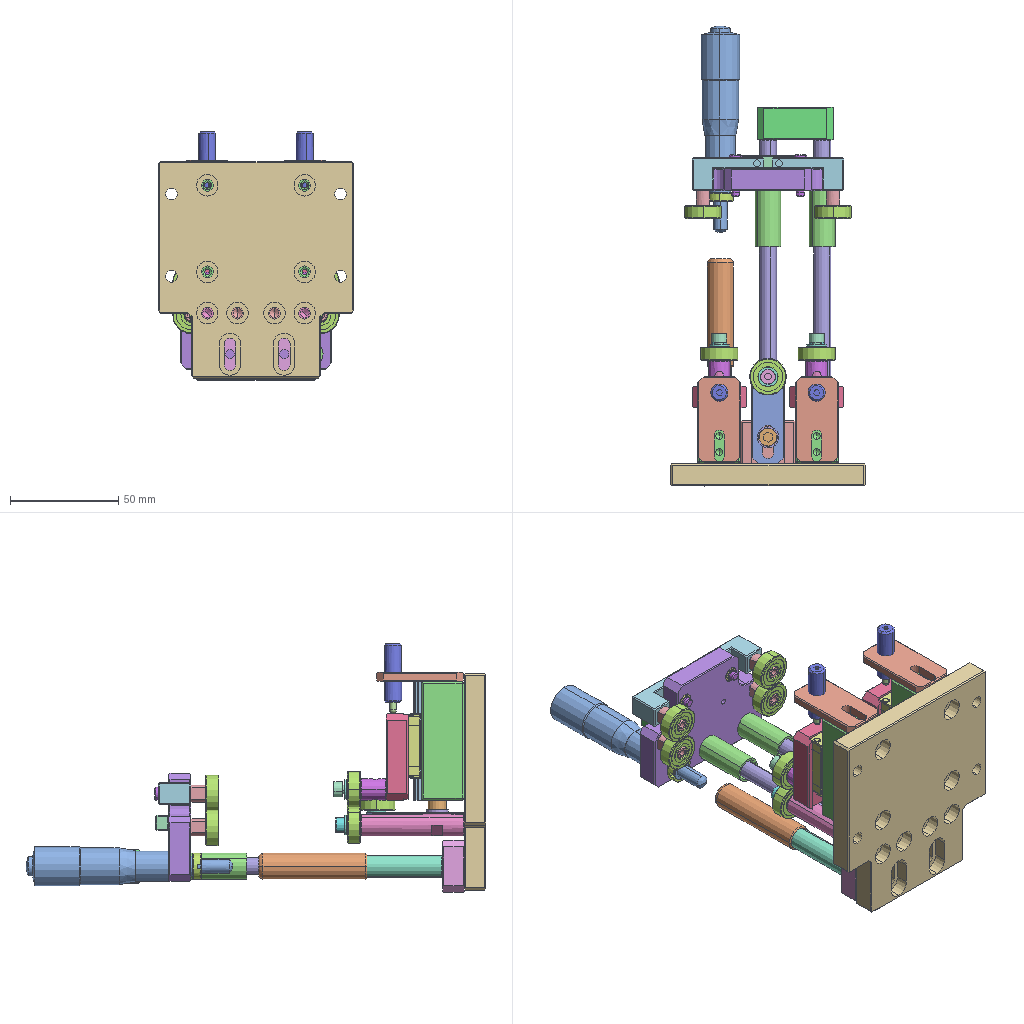Assembly | SolidWorks | 45 different items | 86 placed | box 90 x 212 x 115 mm
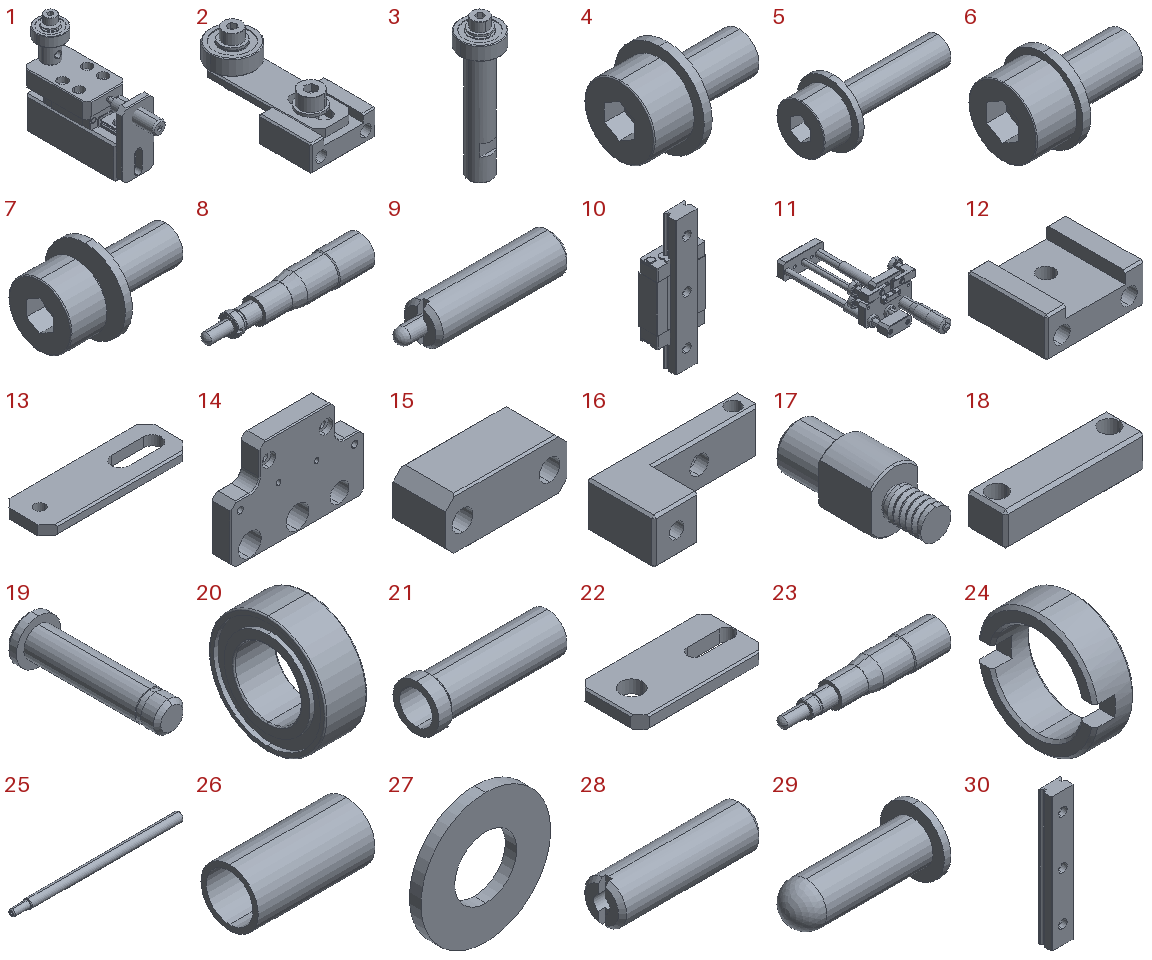Parts list (item | name | quantity | parent item | size | volume | features):
1 | (subassembly) | x2 | - | 25 x 75.736 x 60.345 mm | 39724 mm3 | -
2 | (subassembly) | x1 | - | 25 x 50.976 x 21.6 mm | 7360 mm3 | -
3 | (subassembly) | x2 | - | 17 x 17 x 59.3 mm | 5007 mm3 | -
4 | (subassembly) | x2 | in 3 | 12 x 9 x 9 mm | 278.436 mm3 | -
5 | (subassembly) | x1 | in 2 | 20 x 9 x 9 mm | 378.967 mm3 | -
6 | (subassembly) | x1 | in 2 | 15 x 10 x 10 mm | 502.571 mm3 | -
7 | (subassembly) | x2 | in 1 | 14 x 9 x 9 mm | 303.569 mm3 | -
8 | (subassembly) | x1 | in 11 | 95.5 x 18 x 18 mm | 15301 mm3 | -
9 | (subassembly) | x2 | in 1 | 32 x 8 x 8 mm | 1008 mm3 | -
10 | (subassembly) | x2 | in 1 | 20 x 10 x 55 mm | 5673 mm3 | -
11 | (subassembly) | x1 | - | 77 x 202.46 x 55 mm | 99143 mm3 | features CompositeCurve 4, MateUpdatePoint 3
12 | - | x1 | in 2 | 25 x 20 x 10 mm | 3625 mm3 | features HoleWzd 2, Chamfer 1, Extrusion 1, ICE 1
13 | - | x1 | in 2 | 45 x 15 x 3 mm | 1689 mm3 | features Chamfer 2, Extrusion 1, HoleWzd 1, ICE 1
14 | - | x1 | in 11 | 70 x 10 x 50 mm | 24960 mm3 | features ICE 5, Chamfer 3, HoleWzd 2, Cut 1, Extrusion 1, Fillet 1
15 | - | x1 | in 11 | 35 x 15 x 15 mm | 6742 mm3 | features Chamfer 2, Extrusion 1, ICE 1
16 | - | x2 | in 11 | 33 x 15 x 10 mm | 2355 mm3 | features ICE 5, Chamfer 1, Extrusion 1, HoleWzd 1, MirrorPattern 1
17 | - | x4 | in 11 | 6 x 18.5 x 8 mm | 437.837 mm3 | features ICE 4, Chamfer 2, Extrusion 1, Helix 1, HoleWzd 1, SweepCut 1
18 | - | x1 | in 11 | 25 x 7 x 6 mm | 851.742 mm3 | features HoleWzd 2, Chamfer 1, Extrusion 1
19 | - | x2 | in 11 | 6 x 19.5 x 6 mm | 263.49 mm3 | features Chamfer 2, Extrusion 1, ICE 1, RevCut 1
20 | - | x4 | in 11 | 2.5 x 7 x 7 mm | 58.917 mm3 | features RefAxis 6, 3DProfileFeature 2, Revolution 1
21 | - | x2 | in 11 | 40 x 14 x 14 mm | 1542 mm3 | features RefAxis 3, 3DProfileFeature 1, Revolution 1
22 | - | x2 | in 1 | 40 x 20 x 4 mm | 2715 mm3 | features Chamfer 2, Extrusion 1, HoleWzd 1, ICE 1
23 | - | x1 | in 8 | 95.5 x 18 x 18 mm | 15118 mm3 | features RefAxis 9, 3DProfileFeature 3, RevCut 1, Revolution 1
24 | - | x1 | in 8 | 4 x 12 x 12 mm | 182.884 mm3 | features RefAxis 3, 3DProfileFeature 1, ICE 1, Revolution 1
25 | - | x2 | in 11 | 155 x 8 x 8 mm | 7283 mm3 | features BaseBody 1, MoveFace 1
26 | - | x2 | in 11 | 20 x 9.8 x 9.8 mm | 503.283 mm3 | features RefAxis 3, 3DProfileFeature 1, Revolution 1
27 | - | x6 | in 2, 4, 5, 7 | 9 x 0.8 x 9 mm | 39.276 mm3 | features Revolution 1
28 | - | x2 | in 9 | 27 x 8 x 8 mm | 931.32 mm3 | features BaseBody 1
29 | - | x2 | in 9 | 10 x 4.8 x 4.8 mm | 76.851 mm3 | features BaseBody 1
30 | - | x2 | in 10 | 9 x 5.5 x 55 mm | 2182 mm3 | features BaseBody 1
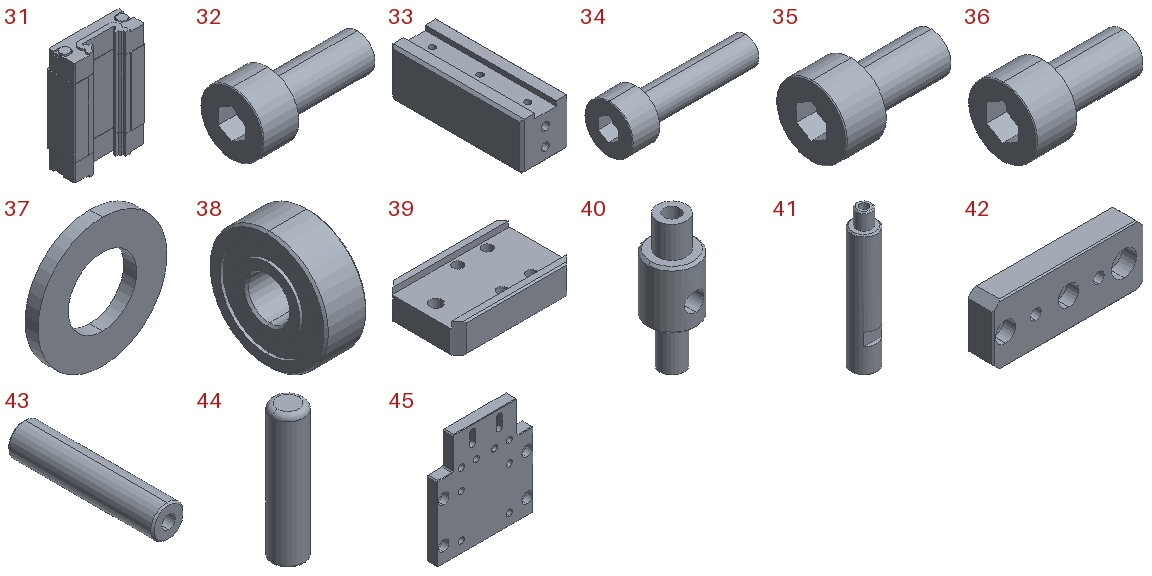31 | - | x2 | in 10 | 20 x 7.8 x 30 mm | 3491 mm3 | features BaseBody 1
32 | - | x2 | in 7 | 14 x 7 x 7 mm | 264.293 mm3 | features BlendCut 1, Cut 1, Fillet 1, LPattern 1, RevCut 1, Revolution 1
33 | - | x2 | in 1 | 20 x 55 x 20 mm | 20279 mm3 | features HoleWzd 3, Chamfer 1, Extrusion 1, ICE 1
34 | - | x1 | in 5 | 20 x 7 x 7 mm | 339.691 mm3 | features BlendCut 1, Cut 1, Fillet 1, LPattern 1, RevCut 1, Revolution 1
35 | - | x2 | in 4 | 12 x 7 x 7 mm | 239.16 mm3 | features BlendCut 1, Cut 1, Fillet 1, LPattern 1, RevCut 1, Revolution 1
36 | - | x1 | in 6 | 15 x 8.5 x 8.5 mm | 446.093 mm3 | features BlendCut 1, Cut 1, Fillet 1, LPattern 1, RevCut 1, Revolution 1
37 | - | x1 | in 6 | 10 x 1 x 10 mm | 56.478 mm3 | features Revolution 1
38 | - | x9 | in 1, 2, 3, 11 | 6 x 17 x 17 mm | 1125 mm3 | features BaseBody 1
39 | - | x2 | in 1 | 40 x 25 x 10 mm | 7537 mm3 | features Chamfer 2, HoleWzd 2, Extrusion 1, ICE 1
40 | - | x2 | in 1 | 10 x 10 x 27.5 mm | 1083 mm3 | features ICE 3, Chamfer 1, Extrusion 1, HoleWzd 1
41 | - | x2 | in 3 | 10 x 10 x 54.5 mm | 3603 mm3 | features HoleWzd 2, ICE 2, Chamfer 1, Extrusion 1, MirrorPattern 1
42 | - | x1 | in 11 | 60 x 10 x 24 mm | 12723 mm3 | features HoleWzd 4, Chamfer 2, Extrusion 1, ICE 1
43 | - | x1 | in 11 | 10 x 45 x 10 mm | 3349 mm3 | features 3DProfileFeature 1, Chamfer 1, Extrusion 1, HoleWzd 1
44 | - | x1 | in 11 | 12 x 12 x 50 mm | 4836 mm3 | features Fillet 2, Extrusion 1, ICE 1
45 | - | x1 | - | 90 x 10 x 100 mm | 71659 mm3 | features HoleWzd 5, Chamfer 2, ICE 2, Extrusion 1
Mates (type | each side: item.copy, entity, surface, feature):
In the top assembly
Coincident | 41.1 face plane Boss-Extrude1 | 45.1 face plane Boss-Extrude1
Coincident | 41.2 face plane Boss-Extrude1 | 45.1 face plane Boss-Extrude1
Width | 12.1 face plane Boss-Extrude1 | 12.1 face plane Boss-Extrude1 | 33.1 face plane Boss-Extrude1 | 33.2 face plane Boss-Extrude1
Coincident | 12.1 face plane Boss-Extrude1 | 45.1 face plane Boss-Extrude1
Coincident | 33.2 face plane Boss-Extrude1 | 45.1 face plane Boss-Extrude1
Coincident | 45.1 face plane Boss-Extrude1 | 42.1 face plane Boss-Extrude1
Parallel | 41.1 face cylinder M5 Tapped Hole1 | 45.1 face cylinder Hole Size (Based On) Socket Head Cap Screw Type2
Concentric | 41.1 face cylinder M5 Tapped Hole1 | 45.1 face cylinder Hole Size (Based On) Socket Head Cap Screw Type2
Concentric | 41.2 face cylinder M5 Tapped Hole1 | 45.1 face cylinder Hole Size (Based On) Socket Head Cap Screw Type2
Concentric | 12.1 face cylinder M5 Tapped Hole2 | 45.1 face cylinder Hole Size (Based On) Socket Head Cap Screw Type2 | 2 times
Concentric | 33.2 face cylinder M5 Tapped Hole1 | 45.1 face cylinder Hole Size (Based On) Socket Head Cap Screw Type2 | 2 times
Concentric | 33.1 face cylinder M5 Tapped Hole1 | 45.1 face cylinder Hole Size (Based On) Socket Head Cap Screw Type2 | 2 times
Parallel | 45.1 plane | assembly plane
Coincident | 45.1 plane | assembly plane
Coincident | 33.1 face plane Boss-Extrude1 | 45.1 face plane Boss-Extrude1
Slot | 42.1 face cylinder M5 Tapped Hole1 | 45.1 face cylinder Hole Size (Based On) Socket Head Cap Screw Type7 | 2 times
In subassembly 2
Coincident | 12.2 face plane Cut-Extrude1 | 13.1 face plane Boss-Extrude1
Parallel | 12.2 face plane Cut-Extrude1 | 13.1 face plane Boss-Extrude1
Slot | 13.1 face plane Cut-Extrude1 | 12.2 face cylinder M5 Tapped Hole1
Concentric | 13.1 face cylinder M4 Tapped Hole1 | 38.1 face cylinder Input1
Concentric | 13.1 face cylinder M4 Tapped Hole1 | 27.1 face cylinder Base-Revolve
Coincident | 13.1 face plane Boss-Extrude1 | 27.1 face plane Base-Revolve
Coincident | 38.1 face plane Input1 | 27.1 face plane Base-Revolve
Concentric | 38.1 face cylinder Input1 | 34.1 face cylinder Base-Revolve
Coincident | 38.1 face plane Input1 | 27.2 face plane Base-Revolve
Concentric | 12.2 face cylinder M5 Tapped Hole1 | 36.1 face cylinder Base-Revolve
Coincident | 13.1 face plane Boss-Extrude1 | 37.1 face plane Base-Revolve
In subassembly 5
Coincident | 34.2 face plane Base-Revolve | 27.1 face plane Base-Revolve
Concentric | 34.2 face cylinder Base-Revolve | 27.1 face cylinder Base-Revolve
In subassembly 6
Concentric | 37.2 face cylinder Base-Revolve | 36.2 face cylinder Base-Revolve
Coincident | 37.2 face plane Base-Revolve | 36.2 face plane Base-Revolve
In subassembly 3
Concentric | 41.3 face cylinder Boss-Extrude2 | 38.1 face cylinder Input1
Coincident | 41.3 face plane Boss-Extrude1 | 38.1 face plane Input1
Concentric | 41.3 face cylinder M4 Tapped Hole1 | 35.1 face cylinder Base-Revolve
Coincident | 41.3 face plane Boss-Extrude2 | 27.3 face plane Base-Revolve
In subassembly 4
Coincident | 35.2 face plane Base-Revolve | 27.1 face plane Base-Revolve
Concentric | 35.2 face cylinder Base-Revolve | 27.1 face cylinder Base-Revolve
In subassembly 1
Coincident | 33.3 face plane Cut-Extrude1 | 30.1 face plane Input1
Concentric | 33.3 face cylinder M3 Tapped Hole1 | 30.1 face cylinder Input1 | 2 times
Coincident | 39.1 face plane Cut-Extrude1 | 31.1 face plane Input1
Concentric | 39.1 face cylinder Hole Size (Based On) Socket Head Cap Screw Type1 | 31.1 face cylinder Input1 | 2 times
Concentric | 39.1 face cylinder M5 Tapped Hole1 | 40.1 face cylinder Boss-Extrude3
Coincident | 39.1 face plane Boss-Extrude1 | 40.1 face plane Boss-Extrude1
Concentric | 40.1 face cylinder Boss-Extrude2 | 38.2 face cylinder Input1
Coincident | 40.1 face plane Boss-Extrude1 | 38.2 face plane Input1
Concentric | 40.1 face cylinder M4 Tapped Hole1 | 32.1 face cylinder Base-Revolve
Coincident | 40.1 face plane Boss-Extrude2 | 27.4 face plane Base-Revolve
Coincident | 33.3 face plane Boss-Extrude1 | 22.1 face plane Boss-Extrude1
Slot | 22.1 face plane Cut-Extrude1 | 33.3 face cylinder M4 Tapped Hole1
Parallel | 33.3 face plane Boss-Extrude1 | 22.1 face plane Boss-Extrude1
Concentric | 22.1 face cylinder M8 Tapped Hole1 | 28.1 face cylinder Input1
In subassembly 7
Concentric | 32.2 face cylinder Base-Revolve | 27.1 face cylinder Base-Revolve
In subassembly 11
Coincident | 14.1 face plane Boss-Extrude1 | 23.1 face plane Revolve1
Concentric | 14.1 face cylinder Cut-Extrude6 | 23.1 face cylinder Revolve1
Concentric | 43.1 face cylinder Boss-Extrude1 | 44.1 face cylinder Cut-Extrude1
Coincident | 43.1 face plane Boss-Extrude1 | 44.1 face plane Cut-Extrude1
Concentric | 25.1 face cylinder Input1 | 26.1 face cylinder Revolve1
Coincident | 42.2 face plane Boss-Extrude1 | 25.1 face plane Input1
Coincident | 42.2 face plane Boss-Extrude1 | 43.1 face plane Boss-Extrude1
Concentric | 25.1 edge | 42.2 edge
Concentric | 25.1 face cylinder Input1 | 21.1 face cylinder Revolve1
Concentric | 25.1 face cylinder Input1 | 15.1 face cylinder Cut-Extrude1
Concentric | 17.1 face cylinder Boss-Extrude2 | 38.1 face cylinder Input1
Concentric | 17.2 face cylinder Boss-Extrude2 | 38.3 face cylinder Input1
Concentric | 14.1 face cylinder M4 Tapped Hole2 | 17.1 face cylinder Boss-Extrude2
Concentric | 14.1 face cylinder M4 Tapped Hole2 | 17.2 edge
Coincident | 38.1 face plane Input1 | 38.3 face plane Input1
Coincident | 17.2 face plane Boss-Extrude1 | 17.1 face plane Boss-Extrude1
Concentric | 14.1 face cylinder Cut-Extrude7 | 21.1 face cylinder Revolve1
Concentric | 23.1 face cylinder Revolve1 | 43.1 face cylinder Boss-Extrude1
Coincident | 14.1 face plane Boss-Extrude1 | 21.1 face plane Revolve1
Coincident | 14.1 face plane Boss-Extrude1 | 17.1 face plane Boss-Extrude1
Concentric | 25.2 face cylinder Input1 | 26.2 face cylinder Revolve1
Concentric | 25.2 face cylinder Input1 | 21.2 face cylinder Revolve1
Coincident | 21.1 face plane Revolve1 | 21.2 face plane Revolve1
Concentric | 14.1 face cylinder Cut-Extrude7 | 21.2 face cylinder Revolve1
Coincident | 14.1 face plane Boss-Extrude1 | 16.1 face plane Cut-Extrude1
Coincident | 17.1 face plane Boss-Extrude2 | 38.1 face plane Input1
Coincident | 16.1 edge | 17.3 face cylinder Boss-Extrude5
Coincident | 17.1 face plane Boss-Extrude1 | 17.3 face plane Boss-Extrude1
Concentric | 17.3 face cylinder Boss-Extrude2 | 38.4 face cylinder Input1
Coincident | 38.1 face plane Input1 | 38.4 face plane Input1
Coincident | 14.1 face plane Boss-Extrude1 | 16.2 face plane Cut-Extrude1
Concentric | 17.4 face cylinder Boss-Extrude2 | 38.5 face cylinder Input1
Coincident | 17.4 face plane Boss-Extrude2 | 38.5 face plane Input1
Concentric | 16.2 face cylinder M4 Tapped Hole1 | 17.4 face cylinder Boss-Extrude2
Coincident | 16.2 face plane Boss-Extrude1 | 17.4 face plane Boss-Extrude1
Coincident | 42.2 face plane Boss-Extrude1 | 25.2 face plane Input1
Coincident | 15.1 face plane Boss-Extrude1 | 25.1 face plane Input1
Concentric | 42.2 face cylinder Hole Size (% Based On) Socket Head Cap Screw Type3 | 25.2 face cylinder Input1
Parallel | 14.1 face plane Boss-Extrude1 | 16.2 face plane Boss-Extrude1
Coincident | 16.1 face plane Boss-Extrude1 | 16.2 face plane Boss-Extrude1
Concentric | 20.1 face cylinder Revolve1 | 19.1 face cylinder Boss-Extrude2
Coincident | 20.1 face plane Revolve1 | 19.1 face plane Boss-Extrude1
Concentric | 16.1 face cylinder Cut-Extrude3 | 20.1 face cylinder Revolve1
Coincident | 16.1 face plane Boss-Extrude1 | 20.1 face plane Revolve1
Concentric | 14.1 face cylinder Cut-Extrude8 | 16.2 face cylinder Cut-Extrude3
Concentric | 14.1 face cylinder Cut-Extrude8 | 16.1 face cylinder Cut-Extrude3
Concentric | 19.2 face cylinder Boss-Extrude2 | 20.2 face cylinder Revolve1
Coincident | 19.2 face plane Boss-Extrude1 | 20.2 face plane Revolve1
Coincident | 16.2 face plane Boss-Extrude1 | 20.2 face plane Revolve1
Concentric | 16.2 face cylinder Cut-Extrude3 | 19.2 face cylinder Boss-Extrude2
Coincident | 14.1 face plane Boss-Extrude1 | 18.1 face plane Boss-Extrude1
Parallel | 14.1 face plane Boss-Extrude2 | 18.1 face plane Boss-Extrude1
Width | 16.1 face plane Boss-Extrude1 | 16.2 face plane Boss-Extrude1 | 18.1 face plane Boss-Extrude1 | 18.1 face plane Boss-Extrude1
DistanceDim | 16.2 face plane Boss-Extrude1 | 18.1 face plane Boss-Extrude1
Coincident | 14.1 face plane Boss-Extrude1 | 20.3 face plane Revolve1
Coincident | 14.1 face plane Boss-Extrude1 | 20.4 face plane Revolve1
Concentric | 19.2 face cylinder Boss-Extrude2 | 20.4 face cylinder Revolve1
Concentric | 19.1 face cylinder Boss-Extrude2 | 20.3 face cylinder Revolve1
In subassembly 8
Coincident | 23.2 plane | 24.1 plane
Coincident | 23.2 axis | 24.1 axis